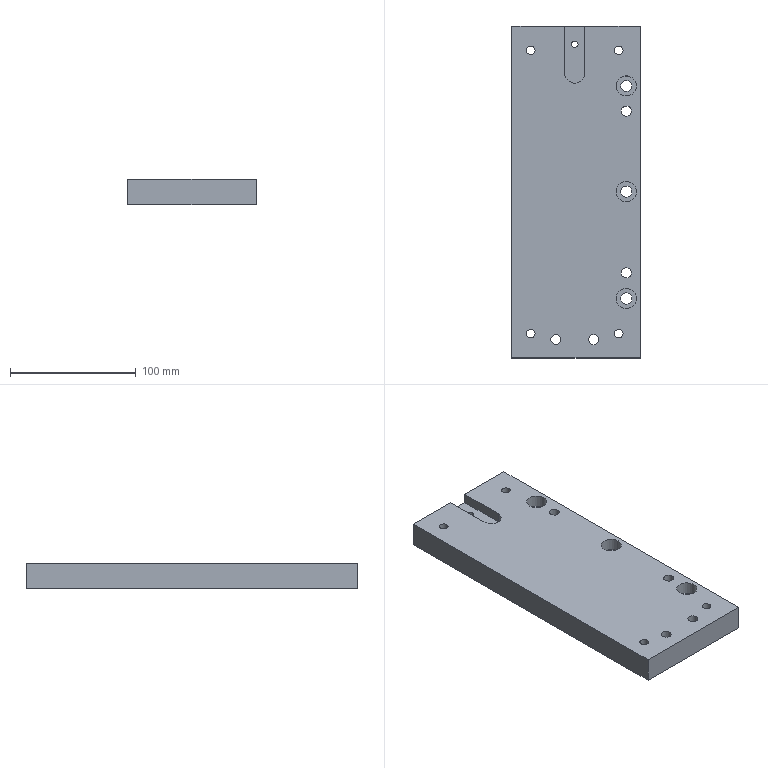Part | NX | features 1605158985 2 | 1 solid | 32 faces | box 102 x 264 x 20 mm | volume 517606 mm3 | cylinder 18 | plane 14 | commonest cylinder face diameters 6.8 x4 8.001 x4 16 x4 9 x3 10.004 x2 5.2 x1
STEP:
#1=CARTESIAN_POINT('',(-383.,131.85,-22.5));
#2=VERTEX_POINT('',#1);
#3=CARTESIAN_POINT('',(-383.,-132.15,-22.5));
#4=VERTEX_POINT('',#3);
#5=CARTESIAN_POINT('',(-383.,38.85,-22.5));
#6=DIRECTION('',(0.,-1.,0.));
#7=VECTOR('',#6,1000.);
#8=LINE('',#5,#7);
#9=EDGE_CURVE('',#2,#4,#8,.T.);
#10=ORIENTED_EDGE('',*,*,#9,.F.);
#11=CARTESIAN_POINT('',(-281.,131.85,-22.5));
#12=VERTEX_POINT('',#11);
#13=CARTESIAN_POINT('',(-303.,131.85,-22.5));
#14=DIRECTION('',(-1.,0.,0.));
#15=VECTOR('',#14,1000.);
#16=LINE('',#13,#15);
#17=EDGE_CURVE('',#12,#2,#16,.T.);
#18=ORIENTED_EDGE('',*,*,#17,.F.);
#19=CARTESIAN_POINT('',(-281.,-132.15,-22.5));
#20=VERTEX_POINT('',#19);
#21=CARTESIAN_POINT('',(-281.,38.85,-22.5));
#22=DIRECTION('',(0.,1.,0.));
#23=VECTOR('',#22,1000.);
#24=LINE('',#21,#23);
#25=EDGE_CURVE('',#20,#12,#24,.T.);
#26=ORIENTED_EDGE('',*,*,#25,.F.);
#27=CARTESIAN_POINT('',(-303.,-132.15,-22.5));
#28=DIRECTION('',(1.,0.,0.));
#29=VECTOR('',#28,1000.);
#30=LINE('',#27,#29);
#31=EDGE_CURVE('',#4,#20,#30,.T.);
#32=ORIENTED_EDGE('',*,*,#31,.F.);
#33=EDGE_LOOP('',(#10,#18,#26,#32));
#34=FACE_BOUND('',#33,.T.);
#35=CARTESIAN_POINT('',(-371.4,112.55,-22.5));
#36=VERTEX_POINT('',#35);
#37=CARTESIAN_POINT('',(-368.,112.55,-22.5));
#38=DIRECTION('',(0.,0.,-1.));
#39=DIRECTION('',(-1.,0.,0.));
#40=AXIS2_PLACEMENT_3D('',#37,#38,#39);
#41=CIRCLE('',#40,3.4);
#42=EDGE_CURVE('',#36,#36,#41,.T.);
#43=ORIENTED_EDGE('',*,*,#42,.F.);
#44=EDGE_LOOP('',(#43));
#45=FACE_BOUND('',#44,.T.);
#46=CARTESIAN_POINT('',(-301.4,112.55,-22.5));
#47=VERTEX_POINT('',#46);
#48=CARTESIAN_POINT('',(-298.,112.55,-22.5));
#49=DIRECTION('',(0.,0.,-1.));
#50=DIRECTION('',(-1.,0.,0.));
#51=AXIS2_PLACEMENT_3D('',#48,#49,#50);
#52=CIRCLE('',#51,3.4);
#53=EDGE_CURVE('',#47,#47,#52,.T.);
#54=ORIENTED_EDGE('',*,*,#53,.F.);
#55=EDGE_LOOP('',(#54));
#56=FACE_BOUND('',#55,.T.);
#57=CARTESIAN_POINT('',(-371.4,-112.85,-22.5));
#58=VERTEX_POINT('',#57);
#59=CARTESIAN_POINT('',(-368.,-112.85,-22.5));
#60=DIRECTION('',(0.,0.,-1.));
#61=DIRECTION('',(-1.,0.,0.));
#62=AXIS2_PLACEMENT_3D('',#59,#60,#61);
#63=CIRCLE('',#62,3.4);
#64=EDGE_CURVE('',#58,#58,#63,.T.);
#65=ORIENTED_EDGE('',*,*,#64,.F.);
#66=EDGE_LOOP('',(#65));
#67=FACE_BOUND('',#66,.T.);
#68=CARTESIAN_POINT('',(-301.4,-112.85,-22.5));
#69=VERTEX_POINT('',#68);
#70=CARTESIAN_POINT('',(-298.,-112.85,-22.5));
#71=DIRECTION('',(0.,0.,-1.));
#72=DIRECTION('',(-1.,0.,0.));
#73=AXIS2_PLACEMENT_3D('',#70,#71,#72);
#74=CIRCLE('',#73,3.4);
#75=EDGE_CURVE('',#69,#69,#74,.T.);
#76=ORIENTED_EDGE('',*,*,#75,.F.);
#77=EDGE_LOOP('',(#76));
#78=FACE_BOUND('',#77,.T.);
#79=CARTESIAN_POINT('',(-296.5,-84.85,-22.5));
#80=VERTEX_POINT('',#79);
#81=CARTESIAN_POINT('',(-292.,-84.85,-22.5));
#82=DIRECTION('',(0.,0.,-1.));
#83=DIRECTION('',(-1.,0.,0.));
#84=AXIS2_PLACEMENT_3D('',#81,#82,#83);
#85=CIRCLE('',#84,4.5);
#86=EDGE_CURVE('',#80,#80,#85,.T.);
#87=ORIENTED_EDGE('',*,*,#86,.F.);
#88=EDGE_LOOP('',(#87));
#89=FACE_BOUND('',#88,.T.);
#90=CARTESIAN_POINT('',(-296.,-64.45,-22.5));
#91=VERTEX_POINT('',#90);
#92=CARTESIAN_POINT('',(-292.,-64.45,-22.5));
#93=DIRECTION('',(0.,0.,-1.));
#94=DIRECTION('',(-1.,0.,0.));
#95=AXIS2_PLACEMENT_3D('',#92,#93,#94);
#96=CIRCLE('',#95,4.);
#97=EDGE_CURVE('',#91,#91,#96,.T.);
#98=ORIENTED_EDGE('',*,*,#97,.F.);
#99=EDGE_LOOP('',(#98));
#100=FACE_BOUND('',#99,.T.);
#101=CARTESIAN_POINT('',(-296.5,0.15,-22.5));
#102=VERTEX_POINT('',#101);
#103=CARTESIAN_POINT('',(-292.,0.15,-22.5));
#104=DIRECTION('',(0.,0.,-1.));
#105=DIRECTION('',(-1.,0.,0.));
#106=AXIS2_PLACEMENT_3D('',#103,#104,#105);
#107=CIRCLE('',#106,4.5);
#108=EDGE_CURVE('',#102,#102,#107,.T.);
#109=ORIENTED_EDGE('',*,*,#108,.F.);
#110=EDGE_LOOP('',(#109));
#111=FACE_BOUND('',#110,.T.);
#112=CARTESIAN_POINT('',(-296.,64.15,-22.5));
#113=VERTEX_POINT('',#112);
#114=CARTESIAN_POINT('',(-292.,64.15,-22.5));
#115=DIRECTION('',(0.,0.,-1.));
#116=DIRECTION('',(-1.,0.,0.));
#117=AXIS2_PLACEMENT_3D('',#114,#115,#116);
#118=CIRCLE('',#117,4.);
#119=EDGE_CURVE('',#113,#113,#118,.T.);
#120=ORIENTED_EDGE('',*,*,#119,.F.);
#121=EDGE_LOOP('',(#120));
#122=FACE_BOUND('',#121,.T.);
#123=CARTESIAN_POINT('',(-296.5,84.15,-22.5));
#124=VERTEX_POINT('',#123);
#125=CARTESIAN_POINT('',(-292.,84.15,-22.5));
#126=DIRECTION('',(0.,0.,-1.));
#127=DIRECTION('',(-1.,0.,0.));
#128=AXIS2_PLACEMENT_3D('',#125,#126,#127);
#129=CIRCLE('',#128,4.5);
#130=EDGE_CURVE('',#124,#124,#129,.T.);
#131=ORIENTED_EDGE('',*,*,#130,.F.);
#132=EDGE_LOOP('',(#131));
#133=FACE_BOUND('',#132,.T.);
#134=CARTESIAN_POINT('',(-353.002,-117.55,-22.5));
#135=VERTEX_POINT('',#134);
#136=CARTESIAN_POINT('',(-348.,-117.55,-22.5));
#137=DIRECTION('',(0.,0.,-1.));
#138=DIRECTION('',(-1.,0.,0.));
#139=AXIS2_PLACEMENT_3D('',#136,#137,#138);
#140=CIRCLE('',#139,5.002);
#141=EDGE_CURVE('',#135,#135,#140,.T.);
#142=ORIENTED_EDGE('',*,*,#141,.F.);
#143=EDGE_LOOP('',(#142));
#144=FACE_BOUND('',#143,.T.);
#145=CARTESIAN_POINT('',(-323.002,-117.55,-22.5));
#146=VERTEX_POINT('',#145);
#147=CARTESIAN_POINT('',(-318.,-117.55,-22.5));
#148=DIRECTION('',(0.,0.,-1.));
#149=DIRECTION('',(-1.,0.,0.));
#150=AXIS2_PLACEMENT_3D('',#147,#148,#149);
#151=CIRCLE('',#150,5.002);
#152=EDGE_CURVE('',#146,#146,#151,.T.);
#153=ORIENTED_EDGE('',*,*,#152,.F.);
#154=EDGE_LOOP('',(#153));
#155=FACE_BOUND('',#154,.T.);
#156=CARTESIAN_POINT('',(-335.6,117.35,-22.5));
#157=VERTEX_POINT('',#156);
#158=CARTESIAN_POINT('',(-333.,117.35,-22.5));
#159=DIRECTION('',(0.,0.,-1.));
#160=DIRECTION('',(-1.,0.,0.));
#161=AXIS2_PLACEMENT_3D('',#158,#159,#160);
#162=CIRCLE('',#161,2.6);
#163=EDGE_CURVE('',#157,#157,#162,.F.);
#164=ORIENTED_EDGE('',*,*,#163,.T.);
#165=EDGE_LOOP('',(#164));
#166=FACE_BOUND('',#165,.T.);
#167=CARTESIAN_POINT('',(-303.,38.85,-22.5));
#168=DIRECTION('',(0.,0.,-1.));
#169=DIRECTION('',(-1.,0.,0.));
#170=AXIS2_PLACEMENT_3D('',#167,#168,#169);
#171=PLANE('',#170);
#172=ADVANCED_FACE('',(#34,#45,#56,#67,#78,#89,#100,#111,#122,#133,#144,#155,#166),#171,.T.);
#173=CARTESIAN_POINT('',(-294.6,-112.85,-2.5));
#174=VERTEX_POINT('',#173);
#175=CARTESIAN_POINT('',(-298.,-112.85,-2.5));
#176=DIRECTION('',(0.,0.,-1.));
#177=DIRECTION('',(1.,0.,0.));
#178=AXIS2_PLACEMENT_3D('',#175,#176,#177);
#179=CIRCLE('',#178,3.4);
#180=EDGE_CURVE('',#174,#174,#179,.T.);
#181=ORIENTED_EDGE('',*,*,#180,.F.);
#182=EDGE_LOOP('',(#181));
#183=FACE_BOUND('',#182,.T.);
#184=ORIENTED_EDGE('',*,*,#75,.T.);
#185=EDGE_LOOP('',(#184));
#186=FACE_BOUND('',#185,.T.);
#187=CARTESIAN_POINT('',(-298.,-112.85,-2.5));
#188=DIRECTION('',(0.,0.,-1.));
#189=DIRECTION('',(1.,0.,0.));
#190=AXIS2_PLACEMENT_3D('',#187,#188,#189);
#191=CYLINDRICAL_SURFACE('',#190,3.4);
#192=ADVANCED_FACE('',(#183,#186),#191,.F.);
#193=CARTESIAN_POINT('',(-364.6,-112.85,-2.5));
#194=VERTEX_POINT('',#193);
#195=CARTESIAN_POINT('',(-368.,-112.85,-2.5));
#196=DIRECTION('',(0.,0.,-1.));
#197=DIRECTION('',(1.,0.,0.));
#198=AXIS2_PLACEMENT_3D('',#195,#196,#197);
#199=CIRCLE('',#198,3.4);
#200=EDGE_CURVE('',#194,#194,#199,.T.);
#201=ORIENTED_EDGE('',*,*,#200,.F.);
#202=EDGE_LOOP('',(#201));
#203=FACE_BOUND('',#202,.T.);
#204=ORIENTED_EDGE('',*,*,#64,.T.);
#205=EDGE_LOOP('',(#204));
#206=FACE_BOUND('',#205,.T.);
#207=CARTESIAN_POINT('',(-368.,-112.85,-2.5));
#208=DIRECTION('',(0.,0.,-1.));
#209=DIRECTION('',(1.,0.,0.));
#210=AXIS2_PLACEMENT_3D('',#207,#208,#209);
#211=CYLINDRICAL_SURFACE('',#210,3.4);
#212=ADVANCED_FACE('',(#203,#206),#211,.F.);
#213=CARTESIAN_POINT('',(-294.6,112.55,-2.5));
#214=VERTEX_POINT('',#213);
#215=CARTESIAN_POINT('',(-298.,112.55,-2.5));
#216=DIRECTION('',(0.,0.,-1.));
#217=DIRECTION('',(1.,0.,0.));
#218=AXIS2_PLACEMENT_3D('',#215,#216,#217);
#219=CIRCLE('',#218,3.4);
#220=EDGE_CURVE('',#214,#214,#219,.T.);
#221=ORIENTED_EDGE('',*,*,#220,.F.);
#222=EDGE_LOOP('',(#221));
#223=FACE_BOUND('',#222,.T.);
#224=ORIENTED_EDGE('',*,*,#53,.T.);
#225=EDGE_LOOP('',(#224));
#226=FACE_BOUND('',#225,.T.);
#227=CARTESIAN_POINT('',(-298.,112.55,-2.5));
#228=DIRECTION('',(0.,0.,-1.));
#229=DIRECTION('',(1.,0.,0.));
#230=AXIS2_PLACEMENT_3D('',#227,#228,#229);
#231=CYLINDRICAL_SURFACE('',#230,3.4);
#232=ADVANCED_FACE('',(#223,#226),#231,.F.);
#233=CARTESIAN_POINT('',(-364.6,112.55,-2.5));
#234=VERTEX_POINT('',#233);
#235=CARTESIAN_POINT('',(-368.,112.55,-2.5));
#236=DIRECTION('',(0.,0.,-1.));
#237=DIRECTION('',(1.,0.,0.));
#238=AXIS2_PLACEMENT_3D('',#235,#236,#237);
#239=CIRCLE('',#238,3.4);
#240=EDGE_CURVE('',#234,#234,#239,.T.);
#241=ORIENTED_EDGE('',*,*,#240,.F.);
#242=EDGE_LOOP('',(#241));
#243=FACE_BOUND('',#242,.T.);
#244=ORIENTED_EDGE('',*,*,#42,.T.);
#245=EDGE_LOOP('',(#244));
#246=FACE_BOUND('',#245,.T.);
#247=CARTESIAN_POINT('',(-368.,112.55,-2.5));
#248=DIRECTION('',(0.,0.,-1.));
#249=DIRECTION('',(1.,0.,0.));
#250=AXIS2_PLACEMENT_3D('',#247,#248,#249);
#251=CYLINDRICAL_SURFACE('',#250,3.4);
#252=ADVANCED_FACE('',(#243,#246),#251,.F.);
#253=CARTESIAN_POINT('',(-341.,131.85,-2.5));
#254=VERTEX_POINT('',#253);
#255=CARTESIAN_POINT('',(-341.,131.85,-10.5));
#256=VERTEX_POINT('',#255);
#257=CARTESIAN_POINT('',(-341.,131.85,2.5));
#258=DIRECTION('',(0.,0.,-1.));
#259=VECTOR('',#258,1000.);
#260=LINE('',#257,#259);
#261=EDGE_CURVE('',#254,#256,#260,.T.);
#262=ORIENTED_EDGE('',*,*,#261,.T.);
#263=CARTESIAN_POINT('',(-325.,131.85,-10.5));
#264=VERTEX_POINT('',#263);
#265=CARTESIAN_POINT('',(-303.,131.85,-10.5));
#266=DIRECTION('',(-1.,0.,0.));
#267=VECTOR('',#266,1000.);
#268=LINE('',#265,#267);
#269=EDGE_CURVE('',#264,#256,#268,.T.);
#270=ORIENTED_EDGE('',*,*,#269,.F.);
#271=CARTESIAN_POINT('',(-325.,131.85,-2.5));
#272=VERTEX_POINT('',#271);
#273=CARTESIAN_POINT('',(-325.,131.85,-35.5));
#274=DIRECTION('',(0.,0.,-1.));
#275=VECTOR('',#274,1000.);
#276=LINE('',#273,#275);
#277=EDGE_CURVE('',#272,#264,#276,.T.);
#278=ORIENTED_EDGE('',*,*,#277,.F.);
#279=CARTESIAN_POINT('',(-281.,131.85,-2.5));
#280=VERTEX_POINT('',#279);
#281=CARTESIAN_POINT('',(-303.,131.85,-2.5));
#282=DIRECTION('',(1.,0.,0.));
#283=VECTOR('',#282,1000.);
#284=LINE('',#281,#283);
#285=EDGE_CURVE('',#272,#280,#284,.T.);
#286=ORIENTED_EDGE('',*,*,#285,.T.);
#287=CARTESIAN_POINT('',(-281.,131.85,-35.5));
#288=DIRECTION('',(0.,0.,1.));
#289=VECTOR('',#288,1000.);
#290=LINE('',#287,#289);
#291=EDGE_CURVE('',#12,#280,#290,.T.);
#292=ORIENTED_EDGE('',*,*,#291,.F.);
#293=ORIENTED_EDGE('',*,*,#17,.T.);
#294=CARTESIAN_POINT('',(-383.,131.85,-2.5));
#295=VERTEX_POINT('',#294);
#296=CARTESIAN_POINT('',(-383.,131.85,-35.5));
#297=DIRECTION('',(0.,0.,1.));
#298=VECTOR('',#297,1000.);
#299=LINE('',#296,#298);
#300=EDGE_CURVE('',#2,#295,#299,.T.);
#301=ORIENTED_EDGE('',*,*,#300,.T.);
#302=CARTESIAN_POINT('',(-303.,131.85,-2.5));
#303=DIRECTION('',(1.,0.,0.));
#304=VECTOR('',#303,1000.);
#305=LINE('',#302,#304);
#306=EDGE_CURVE('',#295,#254,#305,.T.);
#307=ORIENTED_EDGE('',*,*,#306,.T.);
#308=EDGE_LOOP('',(#262,#270,#278,#286,#292,#293,#301,#307));
#309=FACE_BOUND('',#308,.T.);
#310=CARTESIAN_POINT('',(-303.,131.85,-35.5));
#311=DIRECTION('',(0.,1.,0.));
#312=DIRECTION('',(0.,0.,1.));
#313=AXIS2_PLACEMENT_3D('',#310,#311,#312);
#314=PLANE('',#313);
#315=ADVANCED_FACE('',(#309),#314,.T.);
#316=ORIENTED_EDGE('',*,*,#291,.T.);
#317=CARTESIAN_POINT('',(-281.,-132.15,-2.5));
#318=VERTEX_POINT('',#317);
#319=CARTESIAN_POINT('',(-281.,38.85,-2.5));
#320=DIRECTION('',(0.,-1.,0.));
#321=VECTOR('',#320,1000.);
#322=LINE('',#319,#321);
#323=EDGE_CURVE('',#280,#318,#322,.T.);
#324=ORIENTED_EDGE('',*,*,#323,.T.);
#325=CARTESIAN_POINT('',(-281.,-132.15,-35.5));
#326=DIRECTION('',(0.,0.,1.));
#327=VECTOR('',#326,1000.);
#328=LINE('',#325,#327);
#329=EDGE_CURVE('',#20,#318,#328,.T.);
#330=ORIENTED_EDGE('',*,*,#329,.F.);
#331=ORIENTED_EDGE('',*,*,#25,.T.);
#332=EDGE_LOOP('',(#316,#324,#330,#331));
#333=FACE_BOUND('',#332,.T.);
#334=CARTESIAN_POINT('',(-281.,38.85,-35.5));
#335=DIRECTION('',(1.,0.,0.));
#336=DIRECTION('',(0.,0.,-1.));
#337=AXIS2_PLACEMENT_3D('',#334,#335,#336);
#338=PLANE('',#337);
#339=ADVANCED_FACE('',(#333),#338,.T.);
#340=ORIENTED_EDGE('',*,*,#329,.T.);
#341=CARTESIAN_POINT('',(-383.,-132.15,-2.5));
#342=VERTEX_POINT('',#341);
#343=CARTESIAN_POINT('',(-303.,-132.15,-2.5));
#344=DIRECTION('',(-1.,0.,0.));
#345=VECTOR('',#344,1000.);
#346=LINE('',#343,#345);
#347=EDGE_CURVE('',#318,#342,#346,.T.);
#348=ORIENTED_EDGE('',*,*,#347,.T.);
#349=CARTESIAN_POINT('',(-383.,-132.15,-35.5));
#350=DIRECTION('',(0.,0.,1.));
#351=VECTOR('',#350,1000.);
#352=LINE('',#349,#351);
#353=EDGE_CURVE('',#4,#342,#352,.T.);
#354=ORIENTED_EDGE('',*,*,#353,.F.);
#355=ORIENTED_EDGE('',*,*,#31,.T.);
#356=EDGE_LOOP('',(#340,#348,#354,#355));
#357=FACE_BOUND('',#356,.T.);
#358=CARTESIAN_POINT('',(-303.,-132.15,-35.5));
#359=DIRECTION('',(0.,-1.,0.));
#360=DIRECTION('',(0.,0.,-1.));
#361=AXIS2_PLACEMENT_3D('',#358,#359,#360);
#362=PLANE('',#361);
#363=ADVANCED_FACE('',(#357),#362,.T.);
#364=ORIENTED_EDGE('',*,*,#9,.T.);
#365=ORIENTED_EDGE('',*,*,#353,.T.);
#366=CARTESIAN_POINT('',(-383.,38.85,-2.5));
#367=DIRECTION('',(0.,1.,0.));
#368=VECTOR('',#367,1000.);
#369=LINE('',#366,#368);
#370=EDGE_CURVE('',#342,#295,#369,.T.);
#371=ORIENTED_EDGE('',*,*,#370,.T.);
#372=ORIENTED_EDGE('',*,*,#300,.F.);
#373=EDGE_LOOP('',(#364,#365,#371,#372));
#374=FACE_BOUND('',#373,.T.);
#375=CARTESIAN_POINT('',(-383.,38.85,-35.5));
#376=DIRECTION('',(-1.,0.,0.));
#377=DIRECTION('',(0.,0.,1.));
#378=AXIS2_PLACEMENT_3D('',#375,#376,#377);
#379=PLANE('',#378);
#380=ADVANCED_FACE('',(#374),#379,.T.);
#381=ORIENTED_EDGE('',*,*,#285,.F.);
#382=CARTESIAN_POINT('',(-325.,94.35,-2.5));
#383=VERTEX_POINT('',#382);
#384=CARTESIAN_POINT('',(-325.,38.85,-2.5));
#385=DIRECTION('',(0.,1.,0.));
#386=VECTOR('',#385,1000.);
#387=LINE('',#384,#386);
#388=EDGE_CURVE('',#383,#272,#387,.T.);
#389=ORIENTED_EDGE('',*,*,#388,.F.);
#390=CARTESIAN_POINT('',(-341.,94.35,-2.5));
#391=VERTEX_POINT('',#390);
#392=CARTESIAN_POINT('',(-333.,94.35,-2.5));
#393=DIRECTION('',(0.,0.,1.));
#394=DIRECTION('',(1.,0.,0.));
#395=AXIS2_PLACEMENT_3D('',#392,#393,#394);
#396=CIRCLE('',#395,8.);
#397=EDGE_CURVE('',#391,#383,#396,.T.);
#398=ORIENTED_EDGE('',*,*,#397,.F.);
#399=CARTESIAN_POINT('',(-341.,38.85,-2.5));
#400=DIRECTION('',(0.,-1.,0.));
#401=VECTOR('',#400,1000.);
#402=LINE('',#399,#401);
#403=EDGE_CURVE('',#254,#391,#402,.T.);
#404=ORIENTED_EDGE('',*,*,#403,.F.);
#405=ORIENTED_EDGE('',*,*,#306,.F.);
#406=ORIENTED_EDGE('',*,*,#370,.F.);
#407=ORIENTED_EDGE('',*,*,#347,.F.);
#408=ORIENTED_EDGE('',*,*,#323,.F.);
#409=EDGE_LOOP('',(#381,#389,#398,#404,#405,#406,#407,#408));
#410=FACE_BOUND('',#409,.T.);
#411=CARTESIAN_POINT('',(-314.,-117.55,-2.5));
#412=VERTEX_POINT('',#411);
#413=CARTESIAN_POINT('',(-318.,-117.55,-2.5));
#414=DIRECTION('',(0.,0.,1.));
#415=DIRECTION('',(1.,0.,0.));
#416=AXIS2_PLACEMENT_3D('',#413,#414,#415);
#417=CIRCLE('',#416,4.);
#418=EDGE_CURVE('',#412,#412,#417,.T.);
#419=ORIENTED_EDGE('',*,*,#418,.F.);
#420=EDGE_LOOP('',(#419));
#421=FACE_BOUND('',#420,.T.);
#422=CARTESIAN_POINT('',(-344.,-117.55,-2.5));
#423=VERTEX_POINT('',#422);
#424=CARTESIAN_POINT('',(-348.,-117.55,-2.5));
#425=DIRECTION('',(0.,0.,1.));
#426=DIRECTION('',(1.,0.,0.));
#427=AXIS2_PLACEMENT_3D('',#424,#425,#426);
#428=CIRCLE('',#427,4.);
#429=EDGE_CURVE('',#423,#423,#428,.T.);
#430=ORIENTED_EDGE('',*,*,#429,.F.);
#431=EDGE_LOOP('',(#430));
#432=FACE_BOUND('',#431,.T.);
#433=CARTESIAN_POINT('',(-284.,84.15,-2.5));
#434=VERTEX_POINT('',#433);
#435=CARTESIAN_POINT('',(-292.,84.15,-2.5));
#436=DIRECTION('',(0.,0.,1.));
#437=DIRECTION('',(1.,0.,0.));
#438=AXIS2_PLACEMENT_3D('',#435,#436,#437);
#439=CIRCLE('',#438,8.);
#440=EDGE_CURVE('',#434,#434,#439,.T.);
#441=ORIENTED_EDGE('',*,*,#440,.F.);
#442=EDGE_LOOP('',(#441));
#443=FACE_BOUND('',#442,.T.);
#444=CARTESIAN_POINT('',(-288.,64.15,-2.5));
#445=VERTEX_POINT('',#444);
#446=CARTESIAN_POINT('',(-292.,64.15,-2.5));
#447=DIRECTION('',(0.,0.,1.));
#448=DIRECTION('',(1.,0.,0.));
#449=AXIS2_PLACEMENT_3D('',#446,#447,#448);
#450=CIRCLE('',#449,4.);
#451=EDGE_CURVE('',#445,#445,#450,.T.);
#452=ORIENTED_EDGE('',*,*,#451,.F.);
#453=EDGE_LOOP('',(#452));
#454=FACE_BOUND('',#453,.T.);
#455=CARTESIAN_POINT('',(-284.,0.15,-2.5));
#456=VERTEX_POINT('',#455);
#457=CARTESIAN_POINT('',(-292.,0.15,-2.5));
#458=DIRECTION('',(0.,0.,1.));
#459=DIRECTION('',(1.,0.,0.));
#460=AXIS2_PLACEMENT_3D('',#457,#458,#459);
#461=CIRCLE('',#460,8.);
#462=EDGE_CURVE('',#456,#456,#461,.T.);
#463=ORIENTED_EDGE('',*,*,#462,.F.);
#464=EDGE_LOOP('',(#463));
#465=FACE_BOUND('',#464,.T.);
#466=CARTESIAN_POINT('',(-288.,-64.45,-2.5));
#467=VERTEX_POINT('',#466);
#468=CARTESIAN_POINT('',(-292.,-64.45,-2.5));
#469=DIRECTION('',(0.,0.,1.));
#470=DIRECTION('',(1.,0.,0.));
#471=AXIS2_PLACEMENT_3D('',#468,#469,#470);
#472=CIRCLE('',#471,4.);
#473=EDGE_CURVE('',#467,#467,#472,.T.);
#474=ORIENTED_EDGE('',*,*,#473,.F.);
#475=EDGE_LOOP('',(#474));
#476=FACE_BOUND('',#475,.T.);
#477=CARTESIAN_POINT('',(-284.,-84.85,-2.5));
#478=VERTEX_POINT('',#477);
#479=CARTESIAN_POINT('',(-292.,-84.85,-2.5));
#480=DIRECTION('',(0.,0.,1.));
#481=DIRECTION('',(1.,0.,0.));
#482=AXIS2_PLACEMENT_3D('',#479,#480,#481);
#483=CIRCLE('',#482,8.);
#484=EDGE_CURVE('',#478,#478,#483,.T.);
#485=ORIENTED_EDGE('',*,*,#484,.F.);
#486=EDGE_LOOP('',(#485));
#487=FACE_BOUND('',#486,.T.);
#488=ORIENTED_EDGE('',*,*,#180,.T.);
#489=EDGE_LOOP('',(#488));
#490=FACE_BOUND('',#489,.T.);
#491=ORIENTED_EDGE('',*,*,#200,.T.);
#492=EDGE_LOOP('',(#491));
#493=FACE_BOUND('',#492,.T.);
#494=ORIENTED_EDGE('',*,*,#240,.T.);
#495=EDGE_LOOP('',(#494));
#496=FACE_BOUND('',#495,.T.);
#497=ORIENTED_EDGE('',*,*,#220,.T.);
#498=EDGE_LOOP('',(#497));
#499=FACE_BOUND('',#498,.T.);
#500=CARTESIAN_POINT('',(-303.,38.85,-2.5));
#501=DIRECTION('',(0.,0.,1.));
#502=DIRECTION('',(1.,0.,0.));
#503=AXIS2_PLACEMENT_3D('',#500,#501,#502);
#504=PLANE('',#503);
#505=ADVANCED_FACE('',(#410,#421,#432,#443,#454,#465,#476,#487,#490,#493,#496,#499),#504,.T.);
#506=ORIENTED_EDGE('',*,*,#86,.T.);
#507=EDGE_LOOP('',(#506));
#508=FACE_BOUND('',#507,.T.);
#509=CARTESIAN_POINT('',(-296.5,-84.85,-12.5));
#510=VERTEX_POINT('',#509);
#511=CARTESIAN_POINT('',(-292.,-84.85,-12.5));
#512=DIRECTION('',(0.,0.,-1.));
#513=DIRECTION('',(-1.,0.,0.));
#514=AXIS2_PLACEMENT_3D('',#511,#512,#513);
#515=CIRCLE('',#514,4.5);
#516=EDGE_CURVE('',#510,#510,#515,.F.);
#517=ORIENTED_EDGE('',*,*,#516,.T.);
#518=EDGE_LOOP('',(#517));
#519=FACE_BOUND('',#518,.T.);
#520=CARTESIAN_POINT('',(-292.,-84.85,-51.5));
#521=DIRECTION('',(0.,0.,1.));
#522=DIRECTION('',(1.,0.,0.));
#523=AXIS2_PLACEMENT_3D('',#520,#521,#522);
#524=CYLINDRICAL_SURFACE('',#523,4.5);
#525=ADVANCED_FACE('',(#508,#519),#524,.F.);
#526=CARTESIAN_POINT('',(-300.,-84.85,-12.5));
#527=VERTEX_POINT('',#526);
#528=CARTESIAN_POINT('',(-292.,-84.85,-12.5));
#529=DIRECTION('',(0.,0.,-1.));
#530=DIRECTION('',(-1.,0.,0.));
#531=AXIS2_PLACEMENT_3D('',#528,#529,#530);
#532=CIRCLE('',#531,8.);
#533=EDGE_CURVE('',#527,#527,#532,.T.);
#534=ORIENTED_EDGE('',*,*,#533,.F.);
#535=EDGE_LOOP('',(#534));
#536=FACE_BOUND('',#535,.T.);
#537=ORIENTED_EDGE('',*,*,#516,.F.);
#538=EDGE_LOOP('',(#537));
#539=FACE_BOUND('',#538,.T.);
#540=CARTESIAN_POINT('',(-292.,-84.85,-12.5));
#541=DIRECTION('',(0.,0.,-1.));
#542=DIRECTION('',(-1.,0.,0.));
#543=AXIS2_PLACEMENT_3D('',#540,#541,#542);
#544=PLANE('',#543);
#545=ADVANCED_FACE('',(#536,#539),#544,.F.);
#546=ORIENTED_EDGE('',*,*,#484,.T.);
#547=EDGE_LOOP('',(#546));
#548=FACE_BOUND('',#547,.T.);
#549=ORIENTED_EDGE('',*,*,#533,.T.);
#550=EDGE_LOOP('',(#549));
#551=FACE_BOUND('',#550,.T.);
#552=CARTESIAN_POINT('',(-292.,-84.85,-31.5));
#553=DIRECTION('',(0.,0.,1.));
#554=DIRECTION('',(1.,0.,0.));
#555=AXIS2_PLACEMENT_3D('',#552,#553,#554);
#556=CYLINDRICAL_SURFACE('',#555,8.);
#557=ADVANCED_FACE('',(#548,#551),#556,.F.);
#558=ORIENTED_EDGE('',*,*,#97,.T.);
#559=EDGE_LOOP('',(#558));
#560=FACE_BOUND('',#559,.T.);
#561=ORIENTED_EDGE('',*,*,#473,.T.);
#562=EDGE_LOOP('',(#561));
#563=FACE_BOUND('',#562,.T.);
#564=CARTESIAN_POINT('',(-292.,-64.45,-51.5));
#565=DIRECTION('',(0.,0.,1.));
#566=DIRECTION('',(1.,0.,0.));
#567=AXIS2_PLACEMENT_3D('',#564,#565,#566);
#568=CYLINDRICAL_SURFACE('',#567,4.);
#569=ADVANCED_FACE('',(#560,#563),#568,.F.);
#570=ORIENTED_EDGE('',*,*,#108,.T.);
#571=EDGE_LOOP('',(#570));
#572=FACE_BOUND('',#571,.T.);
#573=CARTESIAN_POINT('',(-296.5,0.15,-12.5));
#574=VERTEX_POINT('',#573);
#575=CARTESIAN_POINT('',(-292.,0.15,-12.5));
#576=DIRECTION('',(0.,0.,-1.));
#577=DIRECTION('',(-1.,0.,0.));
#578=AXIS2_PLACEMENT_3D('',#575,#576,#577);
#579=CIRCLE('',#578,4.5);
#580=EDGE_CURVE('',#574,#574,#579,.F.);
#581=ORIENTED_EDGE('',*,*,#580,.T.);
#582=EDGE_LOOP('',(#581));
#583=FACE_BOUND('',#582,.T.);
#584=CARTESIAN_POINT('',(-292.,0.15,-51.5));
#585=DIRECTION('',(0.,0.,1.));
#586=DIRECTION('',(1.,0.,0.));
#587=AXIS2_PLACEMENT_3D('',#584,#585,#586);
#588=CYLINDRICAL_SURFACE('',#587,4.5);
#589=ADVANCED_FACE('',(#572,#583),#588,.F.);
#590=CARTESIAN_POINT('',(-300.,0.15,-12.5));
#591=VERTEX_POINT('',#590);
#592=CARTESIAN_POINT('',(-292.,0.15,-12.5));
#593=DIRECTION('',(0.,0.,-1.));
#594=DIRECTION('',(-1.,0.,0.));
#595=AXIS2_PLACEMENT_3D('',#592,#593,#594);
#596=CIRCLE('',#595,8.);
#597=EDGE_CURVE('',#591,#591,#596,.T.);
#598=ORIENTED_EDGE('',*,*,#597,.F.);
#599=EDGE_LOOP('',(#598));
#600=FACE_BOUND('',#599,.T.);
#601=ORIENTED_EDGE('',*,*,#580,.F.);
#602=EDGE_LOOP('',(#601));
#603=FACE_BOUND('',#602,.T.);
#604=CARTESIAN_POINT('',(-292.,0.15,-12.5));
#605=DIRECTION('',(0.,0.,-1.));
#606=DIRECTION('',(-1.,0.,0.));
#607=AXIS2_PLACEMENT_3D('',#604,#605,#606);
#608=PLANE('',#607);
#609=ADVANCED_FACE('',(#600,#603),#608,.F.);
#610=ORIENTED_EDGE('',*,*,#462,.T.);
#611=EDGE_LOOP('',(#610));
#612=FACE_BOUND('',#611,.T.);
#613=ORIENTED_EDGE('',*,*,#597,.T.);
#614=EDGE_LOOP('',(#613));
#615=FACE_BOUND('',#614,.T.);
#616=CARTESIAN_POINT('',(-292.,0.15,-31.5));
#617=DIRECTION('',(0.,0.,1.));
#618=DIRECTION('',(1.,0.,0.));
#619=AXIS2_PLACEMENT_3D('',#616,#617,#618);
#620=CYLINDRICAL_SURFACE('',#619,8.);
#621=ADVANCED_FACE('',(#612,#615),#620,.F.);
#622=ORIENTED_EDGE('',*,*,#119,.T.);
#623=EDGE_LOOP('',(#622));
#624=FACE_BOUND('',#623,.T.);
#625=ORIENTED_EDGE('',*,*,#451,.T.);
#626=EDGE_LOOP('',(#625));
#627=FACE_BOUND('',#626,.T.);
#628=CARTESIAN_POINT('',(-292.,64.15,-51.5));
#629=DIRECTION('',(0.,0.,1.));
#630=DIRECTION('',(1.,0.,0.));
#631=AXIS2_PLACEMENT_3D('',#628,#629,#630);
#632=CYLINDRICAL_SURFACE('',#631,4.);
#633=ADVANCED_FACE('',(#624,#627),#632,.F.);
#634=ORIENTED_EDGE('',*,*,#130,.T.);
#635=EDGE_LOOP('',(#634));
#636=FACE_BOUND('',#635,.T.);
#637=CARTESIAN_POINT('',(-296.5,84.15,-12.5));
#638=VERTEX_POINT('',#637);
#639=CARTESIAN_POINT('',(-292.,84.15,-12.5));
#640=DIRECTION('',(0.,0.,-1.));
#641=DIRECTION('',(-1.,0.,0.));
#642=AXIS2_PLACEMENT_3D('',#639,#640,#641);
#643=CIRCLE('',#642,4.5);
#644=EDGE_CURVE('',#638,#638,#643,.F.);
#645=ORIENTED_EDGE('',*,*,#644,.T.);
#646=EDGE_LOOP('',(#645));
#647=FACE_BOUND('',#646,.T.);
#648=CARTESIAN_POINT('',(-292.,84.15,-51.5));
#649=DIRECTION('',(0.,0.,1.));
#650=DIRECTION('',(1.,0.,0.));
#651=AXIS2_PLACEMENT_3D('',#648,#649,#650);
#652=CYLINDRICAL_SURFACE('',#651,4.5);
#653=ADVANCED_FACE('',(#636,#647),#652,.F.);
#654=CARTESIAN_POINT('',(-300.,84.15,-12.5));
#655=VERTEX_POINT('',#654);
#656=CARTESIAN_POINT('',(-292.,84.15,-12.5));
#657=DIRECTION('',(0.,0.,-1.));
#658=DIRECTION('',(-1.,0.,0.));
#659=AXIS2_PLACEMENT_3D('',#656,#657,#658);
#660=CIRCLE('',#659,8.);
#661=EDGE_CURVE('',#655,#655,#660,.T.);
#662=ORIENTED_EDGE('',*,*,#661,.F.);
#663=EDGE_LOOP('',(#662));
#664=FACE_BOUND('',#663,.T.);
#665=ORIENTED_EDGE('',*,*,#644,.F.);
#666=EDGE_LOOP('',(#665));
#667=FACE_BOUND('',#666,.T.);
#668=CARTESIAN_POINT('',(-292.,84.15,-12.5));
#669=DIRECTION('',(0.,0.,-1.));
#670=DIRECTION('',(-1.,0.,0.));
#671=AXIS2_PLACEMENT_3D('',#668,#669,#670);
#672=PLANE('',#671);
#673=ADVANCED_FACE('',(#664,#667),#672,.F.);
#674=ORIENTED_EDGE('',*,*,#440,.T.);
#675=EDGE_LOOP('',(#674));
#676=FACE_BOUND('',#675,.T.);
#677=ORIENTED_EDGE('',*,*,#661,.T.);
#678=EDGE_LOOP('',(#677));
#679=FACE_BOUND('',#678,.T.);
#680=CARTESIAN_POINT('',(-292.,84.15,-31.5));
#681=DIRECTION('',(0.,0.,1.));
#682=DIRECTION('',(1.,0.,0.));
#683=AXIS2_PLACEMENT_3D('',#680,#681,#682);
#684=CYLINDRICAL_SURFACE('',#683,8.);
#685=ADVANCED_FACE('',(#676,#679),#684,.F.);
#686=ORIENTED_EDGE('',*,*,#429,.T.);
#687=EDGE_LOOP('',(#686));
#688=FACE_BOUND('',#687,.T.);
#689=CARTESIAN_POINT('',(-344.,-117.55,-18.5));
#690=VERTEX_POINT('',#689);
#691=CARTESIAN_POINT('',(-348.,-117.55,-18.5));
#692=DIRECTION('',(0.,0.,1.));
#693=DIRECTION('',(1.,0.,0.));
#694=AXIS2_PLACEMENT_3D('',#691,#692,#693);
#695=CIRCLE('',#694,4.);
#696=EDGE_CURVE('',#690,#690,#695,.F.);
#697=ORIENTED_EDGE('',*,*,#696,.T.);
#698=EDGE_LOOP('',(#697));
#699=FACE_BOUND('',#698,.T.);
#700=CARTESIAN_POINT('',(-348.,-117.55,-2.4));
#701=DIRECTION('',(0.,0.,-1.));
#702=DIRECTION('',(1.,0.,0.));
#703=AXIS2_PLACEMENT_3D('',#700,#701,#702);
#704=CYLINDRICAL_SURFACE('',#703,4.);
#705=ADVANCED_FACE('',(#688,#699),#704,.F.);
#706=CARTESIAN_POINT('',(-342.998,-117.55,-18.5));
#707=VERTEX_POINT('',#706);
#708=CARTESIAN_POINT('',(-348.,-117.55,-18.5));
#709=DIRECTION('',(0.,0.,-1.));
#710=DIRECTION('',(1.,0.,0.));
#711=AXIS2_PLACEMENT_3D('',#708,#709,#710);
#712=CIRCLE('',#711,5.002);
#713=EDGE_CURVE('',#707,#707,#712,.F.);
#714=ORIENTED_EDGE('',*,*,#713,.F.);
#715=EDGE_LOOP('',(#714));
#716=FACE_BOUND('',#715,.T.);
#717=ORIENTED_EDGE('',*,*,#696,.F.);
#718=EDGE_LOOP('',(#717));
#719=FACE_BOUND('',#718,.T.);
#720=CARTESIAN_POINT('',(-348.,-117.55,-18.5));
#721=DIRECTION('',(0.,0.,1.));
#722=DIRECTION('',(1.,0.,0.));
#723=AXIS2_PLACEMENT_3D('',#720,#721,#722);
#724=PLANE('',#723);
#725=ADVANCED_FACE('',(#716,#719),#724,.F.);
#726=ORIENTED_EDGE('',*,*,#141,.T.);
#727=EDGE_LOOP('',(#726));
#728=FACE_BOUND('',#727,.T.);
#729=ORIENTED_EDGE('',*,*,#713,.T.);
#730=EDGE_LOOP('',(#729));
#731=FACE_BOUND('',#730,.T.);
#732=CARTESIAN_POINT('',(-348.,-117.55,-18.5));
#733=DIRECTION('',(0.,0.,-1.));
#734=DIRECTION('',(1.,0.,0.));
#735=AXIS2_PLACEMENT_3D('',#732,#733,#734);
#736=CYLINDRICAL_SURFACE('',#735,5.002);
#737=ADVANCED_FACE('',(#728,#731),#736,.F.);
#738=ORIENTED_EDGE('',*,*,#418,.T.);
#739=EDGE_LOOP('',(#738));
#740=FACE_BOUND('',#739,.T.);
#741=CARTESIAN_POINT('',(-314.,-117.55,-18.5));
#742=VERTEX_POINT('',#741);
#743=CARTESIAN_POINT('',(-318.,-117.55,-18.5));
#744=DIRECTION('',(0.,0.,1.));
#745=DIRECTION('',(1.,0.,0.));
#746=AXIS2_PLACEMENT_3D('',#743,#744,#745);
#747=CIRCLE('',#746,4.);
#748=EDGE_CURVE('',#742,#742,#747,.F.);
#749=ORIENTED_EDGE('',*,*,#748,.T.);
#750=EDGE_LOOP('',(#749));
#751=FACE_BOUND('',#750,.T.);
#752=CARTESIAN_POINT('',(-318.,-117.55,-2.4));
#753=DIRECTION('',(0.,0.,-1.));
#754=DIRECTION('',(1.,0.,0.));
#755=AXIS2_PLACEMENT_3D('',#752,#753,#754);
#756=CYLINDRICAL_SURFACE('',#755,4.);
#757=ADVANCED_FACE('',(#740,#751),#756,.F.);
#758=CARTESIAN_POINT('',(-312.998,-117.55,-18.5));
#759=VERTEX_POINT('',#758);
#760=CARTESIAN_POINT('',(-318.,-117.55,-18.5));
#761=DIRECTION('',(0.,0.,-1.));
#762=DIRECTION('',(1.,0.,0.));
#763=AXIS2_PLACEMENT_3D('',#760,#761,#762);
#764=CIRCLE('',#763,5.002);
#765=EDGE_CURVE('',#759,#759,#764,.F.);
#766=ORIENTED_EDGE('',*,*,#765,.F.);
#767=EDGE_LOOP('',(#766));
#768=FACE_BOUND('',#767,.T.);
#769=ORIENTED_EDGE('',*,*,#748,.F.);
#770=EDGE_LOOP('',(#769));
#771=FACE_BOUND('',#770,.T.);
#772=CARTESIAN_POINT('',(-318.,-117.55,-18.5));
#773=DIRECTION('',(0.,0.,1.));
#774=DIRECTION('',(1.,0.,0.));
#775=AXIS2_PLACEMENT_3D('',#772,#773,#774);
#776=PLANE('',#775);
#777=ADVANCED_FACE('',(#768,#771),#776,.F.);
#778=ORIENTED_EDGE('',*,*,#152,.T.);
#779=EDGE_LOOP('',(#778));
#780=FACE_BOUND('',#779,.T.);
#781=ORIENTED_EDGE('',*,*,#765,.T.);
#782=EDGE_LOOP('',(#781));
#783=FACE_BOUND('',#782,.T.);
#784=CARTESIAN_POINT('',(-318.,-117.55,-18.5));
#785=DIRECTION('',(0.,0.,-1.));
#786=DIRECTION('',(1.,0.,0.));
#787=AXIS2_PLACEMENT_3D('',#784,#785,#786);
#788=CYLINDRICAL_SURFACE('',#787,5.002);
#789=ADVANCED_FACE('',(#780,#783),#788,.F.);
#790=ORIENTED_EDGE('',*,*,#269,.T.);
#791=CARTESIAN_POINT('',(-341.,94.35,-10.5));
#792=VERTEX_POINT('',#791);
#793=CARTESIAN_POINT('',(-341.,110.35,-10.5));
#794=DIRECTION('',(0.,1.,0.));
#795=VECTOR('',#794,1000.);
#796=LINE('',#793,#795);
#797=EDGE_CURVE('',#256,#792,#796,.F.);
#798=ORIENTED_EDGE('',*,*,#797,.T.);
#799=CARTESIAN_POINT('',(-325.,94.35,-10.5));
#800=VERTEX_POINT('',#799);
#801=CARTESIAN_POINT('',(-333.,94.35,-10.5));
#802=DIRECTION('',(0.,0.,-1.));
#803=DIRECTION('',(1.,0.,0.));
#804=AXIS2_PLACEMENT_3D('',#801,#802,#803);
#805=CIRCLE('',#804,8.);
#806=EDGE_CURVE('',#792,#800,#805,.F.);
#807=ORIENTED_EDGE('',*,*,#806,.T.);
#808=CARTESIAN_POINT('',(-325.,110.35,-10.5));
#809=DIRECTION('',(0.,-1.,0.));
#810=VECTOR('',#809,1000.);
#811=LINE('',#808,#810);
#812=EDGE_CURVE('',#800,#264,#811,.F.);
#813=ORIENTED_EDGE('',*,*,#812,.T.);
#814=EDGE_LOOP('',(#790,#798,#807,#813));
#815=FACE_BOUND('',#814,.T.);
#816=CARTESIAN_POINT('',(-330.4,117.35,-10.5));
#817=VERTEX_POINT('',#816);
#818=CARTESIAN_POINT('',(-333.,117.35,-10.5));
#819=DIRECTION('',(0.,0.,-1.));
#820=DIRECTION('',(1.,0.,0.));
#821=AXIS2_PLACEMENT_3D('',#818,#819,#820);
#822=CIRCLE('',#821,2.6);
#823=EDGE_CURVE('',#817,#817,#822,.T.);
#824=ORIENTED_EDGE('',*,*,#823,.T.);
#825=EDGE_LOOP('',(#824));
#826=FACE_BOUND('',#825,.T.);
#827=CARTESIAN_POINT('',(-325.,110.35,-10.5));
#828=DIRECTION('',(0.,0.,-1.));
#829=DIRECTION('',(1.,0.,0.));
#830=AXIS2_PLACEMENT_3D('',#827,#828,#829);
#831=PLANE('',#830);
#832=ADVANCED_FACE('',(#815,#826),#831,.F.);
#833=ORIENTED_EDGE('',*,*,#403,.T.);
#834=CARTESIAN_POINT('',(-341.,94.35,2.5));
#835=DIRECTION('',(0.,0.,-1.));
#836=VECTOR('',#835,1000.);
#837=LINE('',#834,#836);
#838=EDGE_CURVE('',#391,#792,#837,.T.);
#839=ORIENTED_EDGE('',*,*,#838,.T.);
#840=ORIENTED_EDGE('',*,*,#797,.F.);
#841=ORIENTED_EDGE('',*,*,#261,.F.);
#842=EDGE_LOOP('',(#833,#839,#840,#841));
#843=FACE_BOUND('',#842,.T.);
#844=CARTESIAN_POINT('',(-341.,110.35,2.5));
#845=DIRECTION('',(-1.,0.,0.));
#846=DIRECTION('',(0.,0.,-1.));
#847=AXIS2_PLACEMENT_3D('',#844,#845,#846);
#848=PLANE('',#847);
#849=ADVANCED_FACE('',(#843),#848,.F.);
#850=ORIENTED_EDGE('',*,*,#388,.T.);
#851=ORIENTED_EDGE('',*,*,#277,.T.);
#852=ORIENTED_EDGE('',*,*,#812,.F.);
#853=CARTESIAN_POINT('',(-325.,94.35,2.5));
#854=DIRECTION('',(0.,0.,1.));
#855=VECTOR('',#854,1000.);
#856=LINE('',#853,#855);
#857=EDGE_CURVE('',#800,#383,#856,.T.);
#858=ORIENTED_EDGE('',*,*,#857,.T.);
#859=EDGE_LOOP('',(#850,#851,#852,#858));
#860=FACE_BOUND('',#859,.T.);
#861=CARTESIAN_POINT('',(-325.,110.35,2.5));
#862=DIRECTION('',(1.,0.,0.));
#863=DIRECTION('',(0.,0.,1.));
#864=AXIS2_PLACEMENT_3D('',#861,#862,#863);
#865=PLANE('',#864);
#866=ADVANCED_FACE('',(#860),#865,.F.);
#867=ORIENTED_EDGE('',*,*,#397,.T.);
#868=ORIENTED_EDGE('',*,*,#857,.F.);
#869=ORIENTED_EDGE('',*,*,#806,.F.);
#870=ORIENTED_EDGE('',*,*,#838,.F.);
#871=EDGE_LOOP('',(#867,#868,#869,#870));
#872=FACE_BOUND('',#871,.T.);
#873=CARTESIAN_POINT('',(-333.,94.35,2.5));
#874=DIRECTION('',(0.,0.,-1.));
#875=DIRECTION('',(1.,0.,0.));
#876=AXIS2_PLACEMENT_3D('',#873,#874,#875);
#877=CYLINDRICAL_SURFACE('',#876,8.);
#878=ADVANCED_FACE('',(#872),#877,.F.);
#879=ORIENTED_EDGE('',*,*,#163,.F.);
#880=EDGE_LOOP('',(#879));
#881=FACE_BOUND('',#880,.T.);
#882=ORIENTED_EDGE('',*,*,#823,.F.);
#883=EDGE_LOOP('',(#882));
#884=FACE_BOUND('',#883,.T.);
#885=CARTESIAN_POINT('',(-333.,117.35,-8.));
#886=DIRECTION('',(0.,0.,-1.));
#887=DIRECTION('',(1.,0.,0.));
#888=AXIS2_PLACEMENT_3D('',#885,#886,#887);
#889=CYLINDRICAL_SURFACE('',#888,2.6);
#890=ADVANCED_FACE('',(#881,#884),#889,.F.);
#891=CLOSED_SHELL('',(#172,#192,#212,#232,#252,#315,#339,#363,#380,#505,#525,#545,#557,#569,#589,#609,#621,#633,#653,#673,#685,#705,#725,#737,#757,#777,#789,#832,#849,#866,#878,#890));
#892=MANIFOLD_SOLID_BREP('',#891);
#893=(LENGTH_UNIT()NAMED_UNIT(*)SI_UNIT(.MILLI.,.METRE.));
#894=UNCERTAINTY_MEASURE_WITH_UNIT(LENGTH_MEASURE(0.00001),#893,'','');
#895=(NAMED_UNIT(*)PLANE_ANGLE_UNIT()SI_UNIT($,.RADIAN.));
#896=(NAMED_UNIT(*)SI_UNIT($,.STERADIAN.)SOLID_ANGLE_UNIT());
#897=(GEOMETRIC_REPRESENTATION_CONTEXT(3)GLOBAL_UNCERTAINTY_ASSIGNED_CONTEXT((#894))GLOBAL_UNIT_ASSIGNED_CONTEXT((#893,#895,#896))REPRESENTATION_CONTEXT('',''));
#898=ADVANCED_BREP_SHAPE_REPRESENTATION('',(#892),#897);